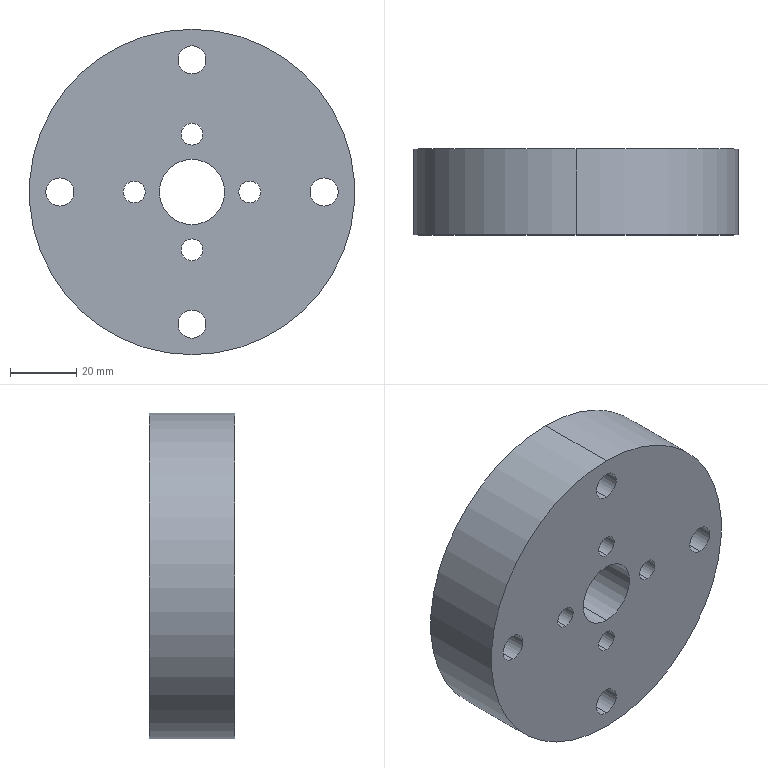Part | SolidWorks | features BaseBody 1 | 1 solid | 34 faces | box 98.5 x 26 x 98.5 mm | volume 179004 mm3 | cylinder 28 | plane 6 | commonest cylinder face diameters 6.6 x8 8.5 x8 11 x8 19.8 x2 98.5 x2
STEP:
#1=CARTESIAN_POINT('',(0.,26.,-49.25));
#2=VERTEX_POINT('',#1);
#3=CARTESIAN_POINT('',(0.,26.,49.25));
#4=VERTEX_POINT('',#3);
#5=CARTESIAN_POINT('',(0.,26.,0.));
#6=DIRECTION('',(0.,-1.,0.));
#7=DIRECTION('',(0.,0.,-1.));
#8=AXIS2_PLACEMENT_3D('',#5,#6,#7);
#9=CIRCLE('',#8,49.25);
#10=EDGE_CURVE('',#2,#4,#9,.T.);
#11=ORIENTED_EDGE('',*,*,#10,.T.);
#12=CARTESIAN_POINT('',(0.,0.,49.25));
#13=VERTEX_POINT('',#12);
#14=CARTESIAN_POINT('',(0.,26.,49.25));
#15=DIRECTION('',(0.,-1.,0.));
#16=VECTOR('',#15,1000.);
#17=LINE('',#14,#16);
#18=EDGE_CURVE('',#4,#13,#17,.T.);
#19=ORIENTED_EDGE('',*,*,#18,.T.);
#20=CARTESIAN_POINT('',(0.,0.,-49.25));
#21=VERTEX_POINT('',#20);
#22=CARTESIAN_POINT('',(0.,0.,0.));
#23=DIRECTION('',(0.,1.,0.));
#24=DIRECTION('',(0.,0.,-1.));
#25=AXIS2_PLACEMENT_3D('',#22,#23,#24);
#26=CIRCLE('',#25,49.25);
#27=EDGE_CURVE('',#13,#21,#26,.T.);
#28=ORIENTED_EDGE('',*,*,#27,.T.);
#29=CARTESIAN_POINT('',(0.,26.,-49.25));
#30=DIRECTION('',(0.,-1.,0.));
#31=VECTOR('',#30,1000.);
#32=LINE('',#29,#31);
#33=EDGE_CURVE('',#2,#21,#32,.T.);
#34=ORIENTED_EDGE('',*,*,#33,.F.);
#35=EDGE_LOOP('',(#11,#19,#28,#34));
#36=FACE_OUTER_BOUND('',#35,.T.);
#37=CARTESIAN_POINT('',(0.,26.,0.));
#38=DIRECTION('',(0.,-1.,0.));
#39=DIRECTION('',(0.,0.,-1.));
#40=AXIS2_PLACEMENT_3D('',#37,#38,#39);
#41=CYLINDRICAL_SURFACE('',#40,49.25);
#42=ADVANCED_FACE('',(#36),#41,.T.);
#43=CARTESIAN_POINT('',(0.,0.,9.9));
#44=VERTEX_POINT('',#43);
#45=CARTESIAN_POINT('',(0.,0.,-9.9));
#46=VERTEX_POINT('',#45);
#47=CARTESIAN_POINT('',(0.,0.,0.));
#48=DIRECTION('',(0.,-1.,0.));
#49=DIRECTION('',(0.,0.,1.));
#50=AXIS2_PLACEMENT_3D('',#47,#48,#49);
#51=CIRCLE('',#50,9.9);
#52=EDGE_CURVE('',#44,#46,#51,.T.);
#53=ORIENTED_EDGE('',*,*,#52,.T.);
#54=CARTESIAN_POINT('',(0.,26.,-9.9));
#55=VERTEX_POINT('',#54);
#56=CARTESIAN_POINT('',(0.,0.,-9.9));
#57=DIRECTION('',(0.,1.,0.));
#58=VECTOR('',#57,1000.);
#59=LINE('',#56,#58);
#60=EDGE_CURVE('',#46,#55,#59,.T.);
#61=ORIENTED_EDGE('',*,*,#60,.T.);
#62=CARTESIAN_POINT('',(0.,26.,9.9));
#63=VERTEX_POINT('',#62);
#64=CARTESIAN_POINT('',(0.,26.,0.));
#65=DIRECTION('',(0.,-1.,0.));
#66=DIRECTION('',(0.,0.,1.));
#67=AXIS2_PLACEMENT_3D('',#64,#65,#66);
#68=CIRCLE('',#67,9.9);
#69=EDGE_CURVE('',#63,#55,#68,.T.);
#70=ORIENTED_EDGE('',*,*,#69,.F.);
#71=CARTESIAN_POINT('',(0.,0.,9.9));
#72=DIRECTION('',(0.,1.,0.));
#73=VECTOR('',#72,1000.);
#74=LINE('',#71,#73);
#75=EDGE_CURVE('',#44,#63,#74,.T.);
#76=ORIENTED_EDGE('',*,*,#75,.F.);
#77=EDGE_LOOP('',(#53,#61,#70,#76));
#78=FACE_OUTER_BOUND('',#77,.T.);
#79=CARTESIAN_POINT('',(0.,0.,0.));
#80=DIRECTION('',(0.,1.,0.));
#81=DIRECTION('',(0.,0.,1.));
#82=AXIS2_PLACEMENT_3D('',#79,#80,#81);
#83=CYLINDRICAL_SURFACE('',#82,9.9);
#84=ADVANCED_FACE('',(#78),#83,.F.);
#85=CARTESIAN_POINT('',(0.,0.,44.25));
#86=VERTEX_POINT('',#85);
#87=CARTESIAN_POINT('',(0.,0.,35.75));
#88=VERTEX_POINT('',#87);
#89=CARTESIAN_POINT('',(0.,0.,40.));
#90=DIRECTION('',(0.,-1.,0.));
#91=DIRECTION('',(0.,0.,1.));
#92=AXIS2_PLACEMENT_3D('',#89,#90,#91);
#93=CIRCLE('',#92,4.25);
#94=EDGE_CURVE('',#86,#88,#93,.T.);
#95=ORIENTED_EDGE('',*,*,#94,.T.);
#96=CARTESIAN_POINT('',(0.,26.,35.75));
#97=VERTEX_POINT('',#96);
#98=CARTESIAN_POINT('',(0.,26.,35.75));
#99=DIRECTION('',(0.,1.,0.));
#100=VECTOR('',#99,1000.);
#101=LINE('',#98,#100);
#102=EDGE_CURVE('',#88,#97,#101,.T.);
#103=ORIENTED_EDGE('',*,*,#102,.T.);
#104=CARTESIAN_POINT('',(0.,26.,44.25));
#105=VERTEX_POINT('',#104);
#106=CARTESIAN_POINT('',(0.,26.,40.));
#107=DIRECTION('',(0.,-1.,0.));
#108=DIRECTION('',(0.,0.,1.));
#109=AXIS2_PLACEMENT_3D('',#106,#107,#108);
#110=CIRCLE('',#109,4.25);
#111=EDGE_CURVE('',#105,#97,#110,.T.);
#112=ORIENTED_EDGE('',*,*,#111,.F.);
#113=CARTESIAN_POINT('',(0.,26.,44.25));
#114=DIRECTION('',(0.,1.,0.));
#115=VECTOR('',#114,1000.);
#116=LINE('',#113,#115);
#117=EDGE_CURVE('',#86,#105,#116,.T.);
#118=ORIENTED_EDGE('',*,*,#117,.F.);
#119=EDGE_LOOP('',(#95,#103,#112,#118));
#120=FACE_OUTER_BOUND('',#119,.T.);
#121=CARTESIAN_POINT('',(0.,26.,40.));
#122=DIRECTION('',(0.,1.,0.));
#123=DIRECTION('',(0.,0.,1.));
#124=AXIS2_PLACEMENT_3D('',#121,#122,#123);
#125=CYLINDRICAL_SURFACE('',#124,4.25);
#126=ADVANCED_FACE('',(#120),#125,.F.);
#127=CARTESIAN_POINT('',(-40.,0.,4.25));
#128=VERTEX_POINT('',#127);
#129=CARTESIAN_POINT('',(-40.,0.,-4.25));
#130=VERTEX_POINT('',#129);
#131=CARTESIAN_POINT('',(-40.,0.,0.));
#132=DIRECTION('',(0.,-1.,0.));
#133=DIRECTION('',(0.,0.,1.));
#134=AXIS2_PLACEMENT_3D('',#131,#132,#133);
#135=CIRCLE('',#134,4.25);
#136=EDGE_CURVE('',#128,#130,#135,.T.);
#137=ORIENTED_EDGE('',*,*,#136,.T.);
#138=CARTESIAN_POINT('',(-40.,26.,-4.25));
#139=VERTEX_POINT('',#138);
#140=CARTESIAN_POINT('',(-40.,26.,-4.25));
#141=DIRECTION('',(0.,1.,0.));
#142=VECTOR('',#141,1000.);
#143=LINE('',#140,#142);
#144=EDGE_CURVE('',#130,#139,#143,.T.);
#145=ORIENTED_EDGE('',*,*,#144,.T.);
#146=CARTESIAN_POINT('',(-40.,26.,4.25));
#147=VERTEX_POINT('',#146);
#148=CARTESIAN_POINT('',(-40.,26.,0.));
#149=DIRECTION('',(0.,-1.,0.));
#150=DIRECTION('',(0.,0.,1.));
#151=AXIS2_PLACEMENT_3D('',#148,#149,#150);
#152=CIRCLE('',#151,4.25);
#153=EDGE_CURVE('',#147,#139,#152,.T.);
#154=ORIENTED_EDGE('',*,*,#153,.F.);
#155=CARTESIAN_POINT('',(-40.,26.,4.25));
#156=DIRECTION('',(0.,1.,0.));
#157=VECTOR('',#156,1000.);
#158=LINE('',#155,#157);
#159=EDGE_CURVE('',#128,#147,#158,.T.);
#160=ORIENTED_EDGE('',*,*,#159,.F.);
#161=EDGE_LOOP('',(#137,#145,#154,#160));
#162=FACE_OUTER_BOUND('',#161,.T.);
#163=CARTESIAN_POINT('',(-40.,26.,0.));
#164=DIRECTION('',(0.,1.,0.));
#165=DIRECTION('',(0.,0.,1.));
#166=AXIS2_PLACEMENT_3D('',#163,#164,#165);
#167=CYLINDRICAL_SURFACE('',#166,4.25);
#168=ADVANCED_FACE('',(#162),#167,.F.);
#169=CARTESIAN_POINT('',(40.,0.,4.25));
#170=VERTEX_POINT('',#169);
#171=CARTESIAN_POINT('',(40.,0.,-4.25));
#172=VERTEX_POINT('',#171);
#173=CARTESIAN_POINT('',(40.,0.,0.));
#174=DIRECTION('',(0.,-1.,0.));
#175=DIRECTION('',(0.,0.,1.));
#176=AXIS2_PLACEMENT_3D('',#173,#174,#175);
#177=CIRCLE('',#176,4.25);
#178=EDGE_CURVE('',#170,#172,#177,.T.);
#179=ORIENTED_EDGE('',*,*,#178,.T.);
#180=CARTESIAN_POINT('',(40.,26.,-4.25));
#181=VERTEX_POINT('',#180);
#182=CARTESIAN_POINT('',(40.,26.,-4.25));
#183=DIRECTION('',(0.,1.,0.));
#184=VECTOR('',#183,1000.);
#185=LINE('',#182,#184);
#186=EDGE_CURVE('',#172,#181,#185,.T.);
#187=ORIENTED_EDGE('',*,*,#186,.T.);
#188=CARTESIAN_POINT('',(40.,26.,4.25));
#189=VERTEX_POINT('',#188);
#190=CARTESIAN_POINT('',(40.,26.,0.));
#191=DIRECTION('',(0.,-1.,0.));
#192=DIRECTION('',(0.,0.,1.));
#193=AXIS2_PLACEMENT_3D('',#190,#191,#192);
#194=CIRCLE('',#193,4.25);
#195=EDGE_CURVE('',#189,#181,#194,.T.);
#196=ORIENTED_EDGE('',*,*,#195,.F.);
#197=CARTESIAN_POINT('',(40.,26.,4.25));
#198=DIRECTION('',(0.,1.,0.));
#199=VECTOR('',#198,1000.);
#200=LINE('',#197,#199);
#201=EDGE_CURVE('',#170,#189,#200,.T.);
#202=ORIENTED_EDGE('',*,*,#201,.F.);
#203=EDGE_LOOP('',(#179,#187,#196,#202));
#204=FACE_OUTER_BOUND('',#203,.T.);
#205=CARTESIAN_POINT('',(40.,26.,0.));
#206=DIRECTION('',(0.,1.,0.));
#207=DIRECTION('',(0.,0.,1.));
#208=AXIS2_PLACEMENT_3D('',#205,#206,#207);
#209=CYLINDRICAL_SURFACE('',#208,4.25);
#210=ADVANCED_FACE('',(#204),#209,.F.);
#211=CARTESIAN_POINT('',(0.,0.,-35.75));
#212=VERTEX_POINT('',#211);
#213=CARTESIAN_POINT('',(0.,0.,-44.25));
#214=VERTEX_POINT('',#213);
#215=CARTESIAN_POINT('',(0.,0.,-40.));
#216=DIRECTION('',(0.,-1.,0.));
#217=DIRECTION('',(0.,0.,1.));
#218=AXIS2_PLACEMENT_3D('',#215,#216,#217);
#219=CIRCLE('',#218,4.25);
#220=EDGE_CURVE('',#212,#214,#219,.T.);
#221=ORIENTED_EDGE('',*,*,#220,.T.);
#222=CARTESIAN_POINT('',(0.,26.,-44.25));
#223=VERTEX_POINT('',#222);
#224=CARTESIAN_POINT('',(0.,26.,-44.25));
#225=DIRECTION('',(0.,1.,0.));
#226=VECTOR('',#225,1000.);
#227=LINE('',#224,#226);
#228=EDGE_CURVE('',#214,#223,#227,.T.);
#229=ORIENTED_EDGE('',*,*,#228,.T.);
#230=CARTESIAN_POINT('',(0.,26.,-35.75));
#231=VERTEX_POINT('',#230);
#232=CARTESIAN_POINT('',(0.,26.,-40.));
#233=DIRECTION('',(0.,-1.,0.));
#234=DIRECTION('',(0.,0.,1.));
#235=AXIS2_PLACEMENT_3D('',#232,#233,#234);
#236=CIRCLE('',#235,4.25);
#237=EDGE_CURVE('',#231,#223,#236,.T.);
#238=ORIENTED_EDGE('',*,*,#237,.F.);
#239=CARTESIAN_POINT('',(0.,26.,-35.75));
#240=DIRECTION('',(0.,1.,0.));
#241=VECTOR('',#240,1000.);
#242=LINE('',#239,#241);
#243=EDGE_CURVE('',#212,#231,#242,.T.);
#244=ORIENTED_EDGE('',*,*,#243,.F.);
#245=EDGE_LOOP('',(#221,#229,#238,#244));
#246=FACE_OUTER_BOUND('',#245,.T.);
#247=CARTESIAN_POINT('',(0.,26.,-40.));
#248=DIRECTION('',(0.,1.,0.));
#249=DIRECTION('',(0.,0.,1.));
#250=AXIS2_PLACEMENT_3D('',#247,#248,#249);
#251=CYLINDRICAL_SURFACE('',#250,4.25);
#252=ADVANCED_FACE('',(#246),#251,.F.);
#253=CARTESIAN_POINT('',(-17.5,0.,3.3));
#254=VERTEX_POINT('',#253);
#255=CARTESIAN_POINT('',(-17.5,0.,-3.3));
#256=VERTEX_POINT('',#255);
#257=CARTESIAN_POINT('',(-17.5,0.,0.));
#258=DIRECTION('',(0.,-1.,0.));
#259=DIRECTION('',(0.,0.,1.));
#260=AXIS2_PLACEMENT_3D('',#257,#258,#259);
#261=CIRCLE('',#260,3.3);
#262=EDGE_CURVE('',#254,#256,#261,.T.);
#263=ORIENTED_EDGE('',*,*,#262,.T.);
#264=CARTESIAN_POINT('',(-17.5,19.2,-3.3));
#265=VERTEX_POINT('',#264);
#266=CARTESIAN_POINT('',(-17.5,26.,-3.3));
#267=DIRECTION('',(0.,1.,0.));
#268=VECTOR('',#267,1000.);
#269=LINE('',#266,#268);
#270=EDGE_CURVE('',#256,#265,#269,.T.);
#271=ORIENTED_EDGE('',*,*,#270,.T.);
#272=CARTESIAN_POINT('',(-17.5,19.2,3.3));
#273=VERTEX_POINT('',#272);
#274=CARTESIAN_POINT('',(-17.5,19.2,0.));
#275=DIRECTION('',(0.,-1.,0.));
#276=DIRECTION('',(0.,0.,1.));
#277=AXIS2_PLACEMENT_3D('',#274,#275,#276);
#278=CIRCLE('',#277,3.3);
#279=EDGE_CURVE('',#273,#265,#278,.T.);
#280=ORIENTED_EDGE('',*,*,#279,.F.);
#281=CARTESIAN_POINT('',(-17.5,26.,3.3));
#282=DIRECTION('',(0.,1.,0.));
#283=VECTOR('',#282,1000.);
#284=LINE('',#281,#283);
#285=EDGE_CURVE('',#254,#273,#284,.T.);
#286=ORIENTED_EDGE('',*,*,#285,.F.);
#287=EDGE_LOOP('',(#263,#271,#280,#286));
#288=FACE_OUTER_BOUND('',#287,.T.);
#289=CARTESIAN_POINT('',(-17.5,26.,0.));
#290=DIRECTION('',(0.,1.,0.));
#291=DIRECTION('',(0.,0.,1.));
#292=AXIS2_PLACEMENT_3D('',#289,#290,#291);
#293=CYLINDRICAL_SURFACE('',#292,3.3);
#294=ADVANCED_FACE('',(#288),#293,.F.);
#295=CARTESIAN_POINT('',(0.,0.,20.8));
#296=VERTEX_POINT('',#295);
#297=CARTESIAN_POINT('',(0.,0.,14.2));
#298=VERTEX_POINT('',#297);
#299=CARTESIAN_POINT('',(0.,0.,17.5));
#300=DIRECTION('',(0.,-1.,0.));
#301=DIRECTION('',(0.,0.,1.));
#302=AXIS2_PLACEMENT_3D('',#299,#300,#301);
#303=CIRCLE('',#302,3.3);
#304=EDGE_CURVE('',#296,#298,#303,.T.);
#305=ORIENTED_EDGE('',*,*,#304,.T.);
#306=CARTESIAN_POINT('',(0.,19.2,14.2));
#307=VERTEX_POINT('',#306);
#308=CARTESIAN_POINT('',(0.,26.,14.2));
#309=DIRECTION('',(0.,1.,0.));
#310=VECTOR('',#309,1000.);
#311=LINE('',#308,#310);
#312=EDGE_CURVE('',#298,#307,#311,.T.);
#313=ORIENTED_EDGE('',*,*,#312,.T.);
#314=CARTESIAN_POINT('',(0.,19.2,20.8));
#315=VERTEX_POINT('',#314);
#316=CARTESIAN_POINT('',(0.,19.2,17.5));
#317=DIRECTION('',(0.,-1.,0.));
#318=DIRECTION('',(0.,0.,1.));
#319=AXIS2_PLACEMENT_3D('',#316,#317,#318);
#320=CIRCLE('',#319,3.3);
#321=EDGE_CURVE('',#315,#307,#320,.T.);
#322=ORIENTED_EDGE('',*,*,#321,.F.);
#323=CARTESIAN_POINT('',(0.,26.,20.8));
#324=DIRECTION('',(0.,1.,0.));
#325=VECTOR('',#324,1000.);
#326=LINE('',#323,#325);
#327=EDGE_CURVE('',#296,#315,#326,.T.);
#328=ORIENTED_EDGE('',*,*,#327,.F.);
#329=EDGE_LOOP('',(#305,#313,#322,#328));
#330=FACE_OUTER_BOUND('',#329,.T.);
#331=CARTESIAN_POINT('',(0.,26.,17.5));
#332=DIRECTION('',(0.,1.,0.));
#333=DIRECTION('',(0.,0.,1.));
#334=AXIS2_PLACEMENT_3D('',#331,#332,#333);
#335=CYLINDRICAL_SURFACE('',#334,3.3);
#336=ADVANCED_FACE('',(#330),#335,.F.);
#337=CARTESIAN_POINT('',(17.5,0.,3.3));
#338=VERTEX_POINT('',#337);
#339=CARTESIAN_POINT('',(17.5,0.,-3.3));
#340=VERTEX_POINT('',#339);
#341=CARTESIAN_POINT('',(17.5,0.,0.));
#342=DIRECTION('',(0.,-1.,0.));
#343=DIRECTION('',(0.,0.,1.));
#344=AXIS2_PLACEMENT_3D('',#341,#342,#343);
#345=CIRCLE('',#344,3.3);
#346=EDGE_CURVE('',#338,#340,#345,.T.);
#347=ORIENTED_EDGE('',*,*,#346,.T.);
#348=CARTESIAN_POINT('',(17.5,19.2,-3.3));
#349=VERTEX_POINT('',#348);
#350=CARTESIAN_POINT('',(17.5,26.,-3.3));
#351=DIRECTION('',(0.,1.,0.));
#352=VECTOR('',#351,1000.);
#353=LINE('',#350,#352);
#354=EDGE_CURVE('',#340,#349,#353,.T.);
#355=ORIENTED_EDGE('',*,*,#354,.T.);
#356=CARTESIAN_POINT('',(17.5,19.2,3.3));
#357=VERTEX_POINT('',#356);
#358=CARTESIAN_POINT('',(17.5,19.2,0.));
#359=DIRECTION('',(0.,-1.,0.));
#360=DIRECTION('',(0.,0.,1.));
#361=AXIS2_PLACEMENT_3D('',#358,#359,#360);
#362=CIRCLE('',#361,3.3);
#363=EDGE_CURVE('',#357,#349,#362,.T.);
#364=ORIENTED_EDGE('',*,*,#363,.F.);
#365=CARTESIAN_POINT('',(17.5,26.,3.3));
#366=DIRECTION('',(0.,1.,0.));
#367=VECTOR('',#366,1000.);
#368=LINE('',#365,#367);
#369=EDGE_CURVE('',#338,#357,#368,.T.);
#370=ORIENTED_EDGE('',*,*,#369,.F.);
#371=EDGE_LOOP('',(#347,#355,#364,#370));
#372=FACE_OUTER_BOUND('',#371,.T.);
#373=CARTESIAN_POINT('',(17.5,26.,0.));
#374=DIRECTION('',(0.,1.,0.));
#375=DIRECTION('',(0.,0.,1.));
#376=AXIS2_PLACEMENT_3D('',#373,#374,#375);
#377=CYLINDRICAL_SURFACE('',#376,3.3);
#378=ADVANCED_FACE('',(#372),#377,.F.);
#379=CARTESIAN_POINT('',(0.,0.,-14.2));
#380=VERTEX_POINT('',#379);
#381=CARTESIAN_POINT('',(0.,0.,-20.8));
#382=VERTEX_POINT('',#381);
#383=CARTESIAN_POINT('',(0.,0.,-17.5));
#384=DIRECTION('',(0.,-1.,0.));
#385=DIRECTION('',(0.,0.,1.));
#386=AXIS2_PLACEMENT_3D('',#383,#384,#385);
#387=CIRCLE('',#386,3.3);
#388=EDGE_CURVE('',#380,#382,#387,.T.);
#389=ORIENTED_EDGE('',*,*,#388,.T.);
#390=CARTESIAN_POINT('',(0.,19.2,-20.8));
#391=VERTEX_POINT('',#390);
#392=CARTESIAN_POINT('',(0.,26.,-20.8));
#393=DIRECTION('',(0.,1.,0.));
#394=VECTOR('',#393,1000.);
#395=LINE('',#392,#394);
#396=EDGE_CURVE('',#382,#391,#395,.T.);
#397=ORIENTED_EDGE('',*,*,#396,.T.);
#398=CARTESIAN_POINT('',(0.,19.2,-14.2));
#399=VERTEX_POINT('',#398);
#400=CARTESIAN_POINT('',(0.,19.2,-17.5));
#401=DIRECTION('',(0.,-1.,0.));
#402=DIRECTION('',(0.,0.,1.));
#403=AXIS2_PLACEMENT_3D('',#400,#401,#402);
#404=CIRCLE('',#403,3.3);
#405=EDGE_CURVE('',#399,#391,#404,.T.);
#406=ORIENTED_EDGE('',*,*,#405,.F.);
#407=CARTESIAN_POINT('',(0.,26.,-14.2));
#408=DIRECTION('',(0.,1.,0.));
#409=VECTOR('',#408,1000.);
#410=LINE('',#407,#409);
#411=EDGE_CURVE('',#380,#399,#410,.T.);
#412=ORIENTED_EDGE('',*,*,#411,.F.);
#413=EDGE_LOOP('',(#389,#397,#406,#412));
#414=FACE_OUTER_BOUND('',#413,.T.);
#415=CARTESIAN_POINT('',(0.,26.,-17.5));
#416=DIRECTION('',(0.,1.,0.));
#417=DIRECTION('',(0.,0.,1.));
#418=AXIS2_PLACEMENT_3D('',#415,#416,#417);
#419=CYLINDRICAL_SURFACE('',#418,3.3);
#420=ADVANCED_FACE('',(#414),#419,.F.);
#421=CARTESIAN_POINT('',(-17.5,19.2,5.5));
#422=VERTEX_POINT('',#421);
#423=CARTESIAN_POINT('',(-17.5,19.2,-5.5));
#424=VERTEX_POINT('',#423);
#425=CARTESIAN_POINT('',(-17.5,19.2,0.));
#426=DIRECTION('',(0.,-1.,0.));
#427=DIRECTION('',(0.,0.,1.));
#428=AXIS2_PLACEMENT_3D('',#425,#426,#427);
#429=CIRCLE('',#428,5.5);
#430=EDGE_CURVE('',#422,#424,#429,.T.);
#431=ORIENTED_EDGE('',*,*,#430,.T.);
#432=CARTESIAN_POINT('',(-17.5,26.,-5.5));
#433=VERTEX_POINT('',#432);
#434=CARTESIAN_POINT('',(-17.5,26.,-5.5));
#435=DIRECTION('',(0.,1.,0.));
#436=VECTOR('',#435,1000.);
#437=LINE('',#434,#436);
#438=EDGE_CURVE('',#424,#433,#437,.T.);
#439=ORIENTED_EDGE('',*,*,#438,.T.);
#440=CARTESIAN_POINT('',(-17.5,26.,5.5));
#441=VERTEX_POINT('',#440);
#442=CARTESIAN_POINT('',(-17.5,26.,0.));
#443=DIRECTION('',(0.,-1.,0.));
#444=DIRECTION('',(0.,0.,1.));
#445=AXIS2_PLACEMENT_3D('',#442,#443,#444);
#446=CIRCLE('',#445,5.5);
#447=EDGE_CURVE('',#441,#433,#446,.T.);
#448=ORIENTED_EDGE('',*,*,#447,.F.);
#449=CARTESIAN_POINT('',(-17.5,26.,5.5));
#450=DIRECTION('',(0.,1.,0.));
#451=VECTOR('',#450,1000.);
#452=LINE('',#449,#451);
#453=EDGE_CURVE('',#422,#441,#452,.T.);
#454=ORIENTED_EDGE('',*,*,#453,.F.);
#455=EDGE_LOOP('',(#431,#439,#448,#454));
#456=FACE_OUTER_BOUND('',#455,.T.);
#457=CARTESIAN_POINT('',(-17.5,26.,0.));
#458=DIRECTION('',(0.,1.,0.));
#459=DIRECTION('',(0.,0.,1.));
#460=AXIS2_PLACEMENT_3D('',#457,#458,#459);
#461=CYLINDRICAL_SURFACE('',#460,5.5);
#462=ADVANCED_FACE('',(#456),#461,.F.);
#463=CARTESIAN_POINT('',(0.,19.2,23.));
#464=VERTEX_POINT('',#463);
#465=CARTESIAN_POINT('',(0.,19.2,12.));
#466=VERTEX_POINT('',#465);
#467=CARTESIAN_POINT('',(0.,19.2,17.5));
#468=DIRECTION('',(0.,-1.,0.));
#469=DIRECTION('',(0.,0.,1.));
#470=AXIS2_PLACEMENT_3D('',#467,#468,#469);
#471=CIRCLE('',#470,5.5);
#472=EDGE_CURVE('',#464,#466,#471,.T.);
#473=ORIENTED_EDGE('',*,*,#472,.T.);
#474=CARTESIAN_POINT('',(0.,26.,12.));
#475=VERTEX_POINT('',#474);
#476=CARTESIAN_POINT('',(0.,26.,12.));
#477=DIRECTION('',(0.,1.,0.));
#478=VECTOR('',#477,1000.);
#479=LINE('',#476,#478);
#480=EDGE_CURVE('',#466,#475,#479,.T.);
#481=ORIENTED_EDGE('',*,*,#480,.T.);
#482=CARTESIAN_POINT('',(0.,26.,23.));
#483=VERTEX_POINT('',#482);
#484=CARTESIAN_POINT('',(0.,26.,17.5));
#485=DIRECTION('',(0.,-1.,0.));
#486=DIRECTION('',(0.,0.,1.));
#487=AXIS2_PLACEMENT_3D('',#484,#485,#486);
#488=CIRCLE('',#487,5.5);
#489=EDGE_CURVE('',#483,#475,#488,.T.);
#490=ORIENTED_EDGE('',*,*,#489,.F.);
#491=CARTESIAN_POINT('',(0.,26.,23.));
#492=DIRECTION('',(0.,1.,0.));
#493=VECTOR('',#492,1000.);
#494=LINE('',#491,#493);
#495=EDGE_CURVE('',#464,#483,#494,.T.);
#496=ORIENTED_EDGE('',*,*,#495,.F.);
#497=EDGE_LOOP('',(#473,#481,#490,#496));
#498=FACE_OUTER_BOUND('',#497,.T.);
#499=CARTESIAN_POINT('',(0.,26.,17.5));
#500=DIRECTION('',(0.,1.,0.));
#501=DIRECTION('',(0.,0.,1.));
#502=AXIS2_PLACEMENT_3D('',#499,#500,#501);
#503=CYLINDRICAL_SURFACE('',#502,5.5);
#504=ADVANCED_FACE('',(#498),#503,.F.);
#505=CARTESIAN_POINT('',(17.5,19.2,5.5));
#506=VERTEX_POINT('',#505);
#507=CARTESIAN_POINT('',(17.5,19.2,-5.5));
#508=VERTEX_POINT('',#507);
#509=CARTESIAN_POINT('',(17.5,19.2,0.));
#510=DIRECTION('',(0.,-1.,0.));
#511=DIRECTION('',(0.,0.,1.));
#512=AXIS2_PLACEMENT_3D('',#509,#510,#511);
#513=CIRCLE('',#512,5.5);
#514=EDGE_CURVE('',#506,#508,#513,.T.);
#515=ORIENTED_EDGE('',*,*,#514,.T.);
#516=CARTESIAN_POINT('',(17.5,26.,-5.5));
#517=VERTEX_POINT('',#516);
#518=CARTESIAN_POINT('',(17.5,26.,-5.5));
#519=DIRECTION('',(0.,1.,0.));
#520=VECTOR('',#519,1000.);
#521=LINE('',#518,#520);
#522=EDGE_CURVE('',#508,#517,#521,.T.);
#523=ORIENTED_EDGE('',*,*,#522,.T.);
#524=CARTESIAN_POINT('',(17.5,26.,5.5));
#525=VERTEX_POINT('',#524);
#526=CARTESIAN_POINT('',(17.5,26.,0.));
#527=DIRECTION('',(0.,-1.,0.));
#528=DIRECTION('',(0.,0.,1.));
#529=AXIS2_PLACEMENT_3D('',#526,#527,#528);
#530=CIRCLE('',#529,5.5);
#531=EDGE_CURVE('',#525,#517,#530,.T.);
#532=ORIENTED_EDGE('',*,*,#531,.F.);
#533=CARTESIAN_POINT('',(17.5,26.,5.5));
#534=DIRECTION('',(0.,1.,0.));
#535=VECTOR('',#534,1000.);
#536=LINE('',#533,#535);
#537=EDGE_CURVE('',#506,#525,#536,.T.);
#538=ORIENTED_EDGE('',*,*,#537,.F.);
#539=EDGE_LOOP('',(#515,#523,#532,#538));
#540=FACE_OUTER_BOUND('',#539,.T.);
#541=CARTESIAN_POINT('',(17.5,26.,0.));
#542=DIRECTION('',(0.,1.,0.));
#543=DIRECTION('',(0.,0.,1.));
#544=AXIS2_PLACEMENT_3D('',#541,#542,#543);
#545=CYLINDRICAL_SURFACE('',#544,5.5);
#546=ADVANCED_FACE('',(#540),#545,.F.);
#547=CARTESIAN_POINT('',(0.,19.2,-12.));
#548=VERTEX_POINT('',#547);
#549=CARTESIAN_POINT('',(0.,19.2,-23.));
#550=VERTEX_POINT('',#549);
#551=CARTESIAN_POINT('',(0.,19.2,-17.5));
#552=DIRECTION('',(0.,-1.,0.));
#553=DIRECTION('',(0.,0.,1.));
#554=AXIS2_PLACEMENT_3D('',#551,#552,#553);
#555=CIRCLE('',#554,5.5);
#556=EDGE_CURVE('',#548,#550,#555,.T.);
#557=ORIENTED_EDGE('',*,*,#556,.T.);
#558=CARTESIAN_POINT('',(0.,26.,-23.));
#559=VERTEX_POINT('',#558);
#560=CARTESIAN_POINT('',(0.,26.,-23.));
#561=DIRECTION('',(0.,1.,0.));
#562=VECTOR('',#561,1000.);
#563=LINE('',#560,#562);
#564=EDGE_CURVE('',#550,#559,#563,.T.);
#565=ORIENTED_EDGE('',*,*,#564,.T.);
#566=CARTESIAN_POINT('',(0.,26.,-12.));
#567=VERTEX_POINT('',#566);
#568=CARTESIAN_POINT('',(0.,26.,-17.5));
#569=DIRECTION('',(0.,-1.,0.));
#570=DIRECTION('',(0.,0.,1.));
#571=AXIS2_PLACEMENT_3D('',#568,#569,#570);
#572=CIRCLE('',#571,5.5);
#573=EDGE_CURVE('',#567,#559,#572,.T.);
#574=ORIENTED_EDGE('',*,*,#573,.F.);
#575=CARTESIAN_POINT('',(0.,26.,-12.));
#576=DIRECTION('',(0.,1.,0.));
#577=VECTOR('',#576,1000.);
#578=LINE('',#575,#577);
#579=EDGE_CURVE('',#548,#567,#578,.T.);
#580=ORIENTED_EDGE('',*,*,#579,.F.);
#581=EDGE_LOOP('',(#557,#565,#574,#580));
#582=FACE_OUTER_BOUND('',#581,.T.);
#583=CARTESIAN_POINT('',(0.,26.,-17.5));
#584=DIRECTION('',(0.,1.,0.));
#585=DIRECTION('',(0.,0.,1.));
#586=AXIS2_PLACEMENT_3D('',#583,#584,#585);
#587=CYLINDRICAL_SURFACE('',#586,5.5);
#588=ADVANCED_FACE('',(#582),#587,.F.);
#589=CARTESIAN_POINT('',(0.,0.,0.));
#590=DIRECTION('',(0.,1.,0.));
#591=DIRECTION('',(0.,0.,-1.));
#592=AXIS2_PLACEMENT_3D('',#589,#590,#591);
#593=CIRCLE('',#592,49.25);
#594=EDGE_CURVE('',#21,#13,#593,.T.);
#595=ORIENTED_EDGE('',*,*,#594,.F.);
#596=ORIENTED_EDGE('',*,*,#27,.F.);
#597=EDGE_LOOP('',(#595,#596));
#598=FACE_OUTER_BOUND('',#597,.T.);
#599=ORIENTED_EDGE('',*,*,#52,.F.);
#600=CARTESIAN_POINT('',(0.,0.,0.));
#601=DIRECTION('',(0.,-1.,0.));
#602=DIRECTION('',(0.,0.,1.));
#603=AXIS2_PLACEMENT_3D('',#600,#601,#602);
#604=CIRCLE('',#603,9.9);
#605=EDGE_CURVE('',#46,#44,#604,.T.);
#606=ORIENTED_EDGE('',*,*,#605,.F.);
#607=EDGE_LOOP('',(#599,#606));
#608=FACE_BOUND('',#607,.T.);
#609=ORIENTED_EDGE('',*,*,#94,.F.);
#610=CARTESIAN_POINT('',(0.,0.,40.));
#611=DIRECTION('',(0.,-1.,0.));
#612=DIRECTION('',(0.,0.,1.));
#613=AXIS2_PLACEMENT_3D('',#610,#611,#612);
#614=CIRCLE('',#613,4.25);
#615=EDGE_CURVE('',#88,#86,#614,.T.);
#616=ORIENTED_EDGE('',*,*,#615,.F.);
#617=EDGE_LOOP('',(#609,#616));
#618=FACE_BOUND('',#617,.T.);
#619=ORIENTED_EDGE('',*,*,#136,.F.);
#620=CARTESIAN_POINT('',(-40.,0.,0.));
#621=DIRECTION('',(0.,-1.,0.));
#622=DIRECTION('',(0.,0.,1.));
#623=AXIS2_PLACEMENT_3D('',#620,#621,#622);
#624=CIRCLE('',#623,4.25);
#625=EDGE_CURVE('',#130,#128,#624,.T.);
#626=ORIENTED_EDGE('',*,*,#625,.F.);
#627=EDGE_LOOP('',(#619,#626));
#628=FACE_BOUND('',#627,.T.);
#629=ORIENTED_EDGE('',*,*,#178,.F.);
#630=CARTESIAN_POINT('',(40.,0.,0.));
#631=DIRECTION('',(0.,-1.,0.));
#632=DIRECTION('',(0.,0.,1.));
#633=AXIS2_PLACEMENT_3D('',#630,#631,#632);
#634=CIRCLE('',#633,4.25);
#635=EDGE_CURVE('',#172,#170,#634,.T.);
#636=ORIENTED_EDGE('',*,*,#635,.F.);
#637=EDGE_LOOP('',(#629,#636));
#638=FACE_BOUND('',#637,.T.);
#639=ORIENTED_EDGE('',*,*,#220,.F.);
#640=CARTESIAN_POINT('',(0.,0.,-40.));
#641=DIRECTION('',(0.,-1.,0.));
#642=DIRECTION('',(0.,0.,1.));
#643=AXIS2_PLACEMENT_3D('',#640,#641,#642);
#644=CIRCLE('',#643,4.25);
#645=EDGE_CURVE('',#214,#212,#644,.T.);
#646=ORIENTED_EDGE('',*,*,#645,.F.);
#647=EDGE_LOOP('',(#639,#646));
#648=FACE_BOUND('',#647,.T.);
#649=ORIENTED_EDGE('',*,*,#262,.F.);
#650=CARTESIAN_POINT('',(-17.5,0.,0.));
#651=DIRECTION('',(0.,-1.,0.));
#652=DIRECTION('',(0.,0.,1.));
#653=AXIS2_PLACEMENT_3D('',#650,#651,#652);
#654=CIRCLE('',#653,3.3);
#655=EDGE_CURVE('',#256,#254,#654,.T.);
#656=ORIENTED_EDGE('',*,*,#655,.F.);
#657=EDGE_LOOP('',(#649,#656));
#658=FACE_BOUND('',#657,.T.);
#659=ORIENTED_EDGE('',*,*,#304,.F.);
#660=CARTESIAN_POINT('',(0.,0.,17.5));
#661=DIRECTION('',(0.,-1.,0.));
#662=DIRECTION('',(0.,0.,1.));
#663=AXIS2_PLACEMENT_3D('',#660,#661,#662);
#664=CIRCLE('',#663,3.3);
#665=EDGE_CURVE('',#298,#296,#664,.T.);
#666=ORIENTED_EDGE('',*,*,#665,.F.);
#667=EDGE_LOOP('',(#659,#666));
#668=FACE_BOUND('',#667,.T.);
#669=ORIENTED_EDGE('',*,*,#346,.F.);
#670=CARTESIAN_POINT('',(17.5,0.,0.));
#671=DIRECTION('',(0.,-1.,0.));
#672=DIRECTION('',(0.,0.,1.));
#673=AXIS2_PLACEMENT_3D('',#670,#671,#672);
#674=CIRCLE('',#673,3.3);
#675=EDGE_CURVE('',#340,#338,#674,.T.);
#676=ORIENTED_EDGE('',*,*,#675,.F.);
#677=EDGE_LOOP('',(#669,#676));
#678=FACE_BOUND('',#677,.T.);
#679=ORIENTED_EDGE('',*,*,#388,.F.);
#680=CARTESIAN_POINT('',(0.,0.,-17.5));
#681=DIRECTION('',(0.,-1.,0.));
#682=DIRECTION('',(0.,0.,1.));
#683=AXIS2_PLACEMENT_3D('',#680,#681,#682);
#684=CIRCLE('',#683,3.3);
#685=EDGE_CURVE('',#382,#380,#684,.T.);
#686=ORIENTED_EDGE('',*,*,#685,.F.);
#687=EDGE_LOOP('',(#679,#686));
#688=FACE_BOUND('',#687,.T.);
#689=CARTESIAN_POINT('',(0.,0.,0.));
#690=DIRECTION('',(0.,1.,0.));
#691=DIRECTION('',(0.,0.,1.));
#692=AXIS2_PLACEMENT_3D('',#689,#690,#691);
#693=PLANE('',#692);
#694=ADVANCED_FACE('',(#598,#608,#618,#628,#638,#648,#658,#668,#678,#688),#693,.F.);
#695=ORIENTED_EDGE('',*,*,#18,.F.);
#696=CARTESIAN_POINT('',(0.,26.,0.));
#697=DIRECTION('',(0.,-1.,0.));
#698=DIRECTION('',(0.,0.,-1.));
#699=AXIS2_PLACEMENT_3D('',#696,#697,#698);
#700=CIRCLE('',#699,49.25);
#701=EDGE_CURVE('',#4,#2,#700,.T.);
#702=ORIENTED_EDGE('',*,*,#701,.T.);
#703=ORIENTED_EDGE('',*,*,#33,.T.);
#704=ORIENTED_EDGE('',*,*,#594,.T.);
#705=EDGE_LOOP('',(#695,#702,#703,#704));
#706=FACE_OUTER_BOUND('',#705,.T.);
#707=CARTESIAN_POINT('',(0.,26.,0.));
#708=DIRECTION('',(0.,-1.,0.));
#709=DIRECTION('',(0.,0.,-1.));
#710=AXIS2_PLACEMENT_3D('',#707,#708,#709);
#711=CYLINDRICAL_SURFACE('',#710,49.25);
#712=ADVANCED_FACE('',(#706),#711,.T.);
#713=ORIENTED_EDGE('',*,*,#60,.F.);
#714=ORIENTED_EDGE('',*,*,#605,.T.);
#715=ORIENTED_EDGE('',*,*,#75,.T.);
#716=CARTESIAN_POINT('',(0.,26.,0.));
#717=DIRECTION('',(0.,-1.,0.));
#718=DIRECTION('',(0.,0.,1.));
#719=AXIS2_PLACEMENT_3D('',#716,#717,#718);
#720=CIRCLE('',#719,9.9);
#721=EDGE_CURVE('',#55,#63,#720,.T.);
#722=ORIENTED_EDGE('',*,*,#721,.F.);
#723=EDGE_LOOP('',(#713,#714,#715,#722));
#724=FACE_OUTER_BOUND('',#723,.T.);
#725=CARTESIAN_POINT('',(0.,0.,0.));
#726=DIRECTION('',(0.,1.,0.));
#727=DIRECTION('',(0.,0.,1.));
#728=AXIS2_PLACEMENT_3D('',#725,#726,#727);
#729=CYLINDRICAL_SURFACE('',#728,9.9);
#730=ADVANCED_FACE('',(#724),#729,.F.);
#731=ORIENTED_EDGE('',*,*,#102,.F.);
#732=ORIENTED_EDGE('',*,*,#615,.T.);
#733=ORIENTED_EDGE('',*,*,#117,.T.);
#734=CARTESIAN_POINT('',(0.,26.,40.));
#735=DIRECTION('',(0.,-1.,0.));
#736=DIRECTION('',(0.,0.,1.));
#737=AXIS2_PLACEMENT_3D('',#734,#735,#736);
#738=CIRCLE('',#737,4.25);
#739=EDGE_CURVE('',#97,#105,#738,.T.);
#740=ORIENTED_EDGE('',*,*,#739,.F.);
#741=EDGE_LOOP('',(#731,#732,#733,#740));
#742=FACE_OUTER_BOUND('',#741,.T.);
#743=CARTESIAN_POINT('',(0.,26.,40.));
#744=DIRECTION('',(0.,1.,0.));
#745=DIRECTION('',(0.,0.,1.));
#746=AXIS2_PLACEMENT_3D('',#743,#744,#745);
#747=CYLINDRICAL_SURFACE('',#746,4.25);
#748=ADVANCED_FACE('',(#742),#747,.F.);
#749=ORIENTED_EDGE('',*,*,#144,.F.);
#750=ORIENTED_EDGE('',*,*,#625,.T.);
#751=ORIENTED_EDGE('',*,*,#159,.T.);
#752=CARTESIAN_POINT('',(-40.,26.,0.));
#753=DIRECTION('',(0.,-1.,0.));
#754=DIRECTION('',(0.,0.,1.));
#755=AXIS2_PLACEMENT_3D('',#752,#753,#754);
#756=CIRCLE('',#755,4.25);
#757=EDGE_CURVE('',#139,#147,#756,.T.);
#758=ORIENTED_EDGE('',*,*,#757,.F.);
#759=EDGE_LOOP('',(#749,#750,#751,#758));
#760=FACE_OUTER_BOUND('',#759,.T.);
#761=CARTESIAN_POINT('',(-40.,26.,0.));
#762=DIRECTION('',(0.,1.,0.));
#763=DIRECTION('',(0.,0.,1.));
#764=AXIS2_PLACEMENT_3D('',#761,#762,#763);
#765=CYLINDRICAL_SURFACE('',#764,4.25);
#766=ADVANCED_FACE('',(#760),#765,.F.);
#767=ORIENTED_EDGE('',*,*,#186,.F.);
#768=ORIENTED_EDGE('',*,*,#635,.T.);
#769=ORIENTED_EDGE('',*,*,#201,.T.);
#770=CARTESIAN_POINT('',(40.,26.,0.));
#771=DIRECTION('',(0.,-1.,0.));
#772=DIRECTION('',(0.,0.,1.));
#773=AXIS2_PLACEMENT_3D('',#770,#771,#772);
#774=CIRCLE('',#773,4.25);
#775=EDGE_CURVE('',#181,#189,#774,.T.);
#776=ORIENTED_EDGE('',*,*,#775,.F.);
#777=EDGE_LOOP('',(#767,#768,#769,#776));
#778=FACE_OUTER_BOUND('',#777,.T.);
#779=CARTESIAN_POINT('',(40.,26.,0.));
#780=DIRECTION('',(0.,1.,0.));
#781=DIRECTION('',(0.,0.,1.));
#782=AXIS2_PLACEMENT_3D('',#779,#780,#781);
#783=CYLINDRICAL_SURFACE('',#782,4.25);
#784=ADVANCED_FACE('',(#778),#783,.F.);
#785=ORIENTED_EDGE('',*,*,#228,.F.);
#786=ORIENTED_EDGE('',*,*,#645,.T.);
#787=ORIENTED_EDGE('',*,*,#243,.T.);
#788=CARTESIAN_POINT('',(0.,26.,-40.));
#789=DIRECTION('',(0.,-1.,0.));
#790=DIRECTION('',(0.,0.,1.));
#791=AXIS2_PLACEMENT_3D('',#788,#789,#790);
#792=CIRCLE('',#791,4.25);
#793=EDGE_CURVE('',#223,#231,#792,.T.);
#794=ORIENTED_EDGE('',*,*,#793,.F.);
#795=EDGE_LOOP('',(#785,#786,#787,#794));
#796=FACE_OUTER_BOUND('',#795,.T.);
#797=CARTESIAN_POINT('',(0.,26.,-40.));
#798=DIRECTION('',(0.,1.,0.));
#799=DIRECTION('',(0.,0.,1.));
#800=AXIS2_PLACEMENT_3D('',#797,#798,#799);
#801=CYLINDRICAL_SURFACE('',#800,4.25);
#802=ADVANCED_FACE('',(#796),#801,.F.);
#803=ORIENTED_EDGE('',*,*,#270,.F.);
#804=ORIENTED_EDGE('',*,*,#655,.T.);
#805=ORIENTED_EDGE('',*,*,#285,.T.);
#806=CARTESIAN_POINT('',(-17.5,19.2,0.));
#807=DIRECTION('',(0.,-1.,0.));
#808=DIRECTION('',(0.,0.,1.));
#809=AXIS2_PLACEMENT_3D('',#806,#807,#808);
#810=CIRCLE('',#809,3.3);
#811=EDGE_CURVE('',#265,#273,#810,.T.);
#812=ORIENTED_EDGE('',*,*,#811,.F.);
#813=EDGE_LOOP('',(#803,#804,#805,#812));
#814=FACE_OUTER_BOUND('',#813,.T.);
#815=CARTESIAN_POINT('',(-17.5,26.,0.));
#816=DIRECTION('',(0.,1.,0.));
#817=DIRECTION('',(0.,0.,1.));
#818=AXIS2_PLACEMENT_3D('',#815,#816,#817);
#819=CYLINDRICAL_SURFACE('',#818,3.3);
#820=ADVANCED_FACE('',(#814),#819,.F.);
#821=ORIENTED_EDGE('',*,*,#312,.F.);
#822=ORIENTED_EDGE('',*,*,#665,.T.);
#823=ORIENTED_EDGE('',*,*,#327,.T.);
#824=CARTESIAN_POINT('',(0.,19.2,17.5));
#825=DIRECTION('',(0.,-1.,0.));
#826=DIRECTION('',(0.,0.,1.));
#827=AXIS2_PLACEMENT_3D('',#824,#825,#826);
#828=CIRCLE('',#827,3.3);
#829=EDGE_CURVE('',#307,#315,#828,.T.);
#830=ORIENTED_EDGE('',*,*,#829,.F.);
#831=EDGE_LOOP('',(#821,#822,#823,#830));
#832=FACE_OUTER_BOUND('',#831,.T.);
#833=CARTESIAN_POINT('',(0.,26.,17.5));
#834=DIRECTION('',(0.,1.,0.));
#835=DIRECTION('',(0.,0.,1.));
#836=AXIS2_PLACEMENT_3D('',#833,#834,#835);
#837=CYLINDRICAL_SURFACE('',#836,3.3);
#838=ADVANCED_FACE('',(#832),#837,.F.);
#839=ORIENTED_EDGE('',*,*,#354,.F.);
#840=ORIENTED_EDGE('',*,*,#675,.T.);
#841=ORIENTED_EDGE('',*,*,#369,.T.);
#842=CARTESIAN_POINT('',(17.5,19.2,0.));
#843=DIRECTION('',(0.,-1.,0.));
#844=DIRECTION('',(0.,0.,1.));
#845=AXIS2_PLACEMENT_3D('',#842,#843,#844);
#846=CIRCLE('',#845,3.3);
#847=EDGE_CURVE('',#349,#357,#846,.T.);
#848=ORIENTED_EDGE('',*,*,#847,.F.);
#849=EDGE_LOOP('',(#839,#840,#841,#848));
#850=FACE_OUTER_BOUND('',#849,.T.);
#851=CARTESIAN_POINT('',(17.5,26.,0.));
#852=DIRECTION('',(0.,1.,0.));
#853=DIRECTION('',(0.,0.,1.));
#854=AXIS2_PLACEMENT_3D('',#851,#852,#853);
#855=CYLINDRICAL_SURFACE('',#854,3.3);
#856=ADVANCED_FACE('',(#850),#855,.F.);
#857=ORIENTED_EDGE('',*,*,#396,.F.);
#858=ORIENTED_EDGE('',*,*,#685,.T.);
#859=ORIENTED_EDGE('',*,*,#411,.T.);
#860=CARTESIAN_POINT('',(0.,19.2,-17.5));
#861=DIRECTION('',(0.,-1.,0.));
#862=DIRECTION('',(0.,0.,1.));
#863=AXIS2_PLACEMENT_3D('',#860,#861,#862);
#864=CIRCLE('',#863,3.3);
#865=EDGE_CURVE('',#391,#399,#864,.T.);
#866=ORIENTED_EDGE('',*,*,#865,.F.);
#867=EDGE_LOOP('',(#857,#858,#859,#866));
#868=FACE_OUTER_BOUND('',#867,.T.);
#869=CARTESIAN_POINT('',(0.,26.,-17.5));
#870=DIRECTION('',(0.,1.,0.));
#871=DIRECTION('',(0.,0.,1.));
#872=AXIS2_PLACEMENT_3D('',#869,#870,#871);
#873=CYLINDRICAL_SURFACE('',#872,3.3);
#874=ADVANCED_FACE('',(#868),#873,.F.);
#875=ORIENTED_EDGE('',*,*,#10,.F.);
#876=ORIENTED_EDGE('',*,*,#701,.F.);
#877=EDGE_LOOP('',(#875,#876));
#878=FACE_OUTER_BOUND('',#877,.T.);
#879=ORIENTED_EDGE('',*,*,#69,.T.);
#880=ORIENTED_EDGE('',*,*,#721,.T.);
#881=EDGE_LOOP('',(#879,#880));
#882=FACE_BOUND('',#881,.T.);
#883=ORIENTED_EDGE('',*,*,#111,.T.);
#884=ORIENTED_EDGE('',*,*,#739,.T.);
#885=EDGE_LOOP('',(#883,#884));
#886=FACE_BOUND('',#885,.T.);
#887=ORIENTED_EDGE('',*,*,#153,.T.);
#888=ORIENTED_EDGE('',*,*,#757,.T.);
#889=EDGE_LOOP('',(#887,#888));
#890=FACE_BOUND('',#889,.T.);
#891=ORIENTED_EDGE('',*,*,#195,.T.);
#892=ORIENTED_EDGE('',*,*,#775,.T.);
#893=EDGE_LOOP('',(#891,#892));
#894=FACE_BOUND('',#893,.T.);
#895=ORIENTED_EDGE('',*,*,#237,.T.);
#896=ORIENTED_EDGE('',*,*,#793,.T.);
#897=EDGE_LOOP('',(#895,#896));
#898=FACE_BOUND('',#897,.T.);
#899=ORIENTED_EDGE('',*,*,#447,.T.);
#900=CARTESIAN_POINT('',(-17.5,26.,0.));
#901=DIRECTION('',(0.,-1.,0.));
#902=DIRECTION('',(0.,0.,1.));
#903=AXIS2_PLACEMENT_3D('',#900,#901,#902);
#904=CIRCLE('',#903,5.5);
#905=EDGE_CURVE('',#433,#441,#904,.T.);
#906=ORIENTED_EDGE('',*,*,#905,.T.);
#907=EDGE_LOOP('',(#899,#906));
#908=FACE_BOUND('',#907,.T.);
#909=ORIENTED_EDGE('',*,*,#489,.T.);
#910=CARTESIAN_POINT('',(0.,26.,17.5));
#911=DIRECTION('',(0.,-1.,0.));
#912=DIRECTION('',(0.,0.,1.));
#913=AXIS2_PLACEMENT_3D('',#910,#911,#912);
#914=CIRCLE('',#913,5.5);
#915=EDGE_CURVE('',#475,#483,#914,.T.);
#916=ORIENTED_EDGE('',*,*,#915,.T.);
#917=EDGE_LOOP('',(#909,#916));
#918=FACE_BOUND('',#917,.T.);
#919=ORIENTED_EDGE('',*,*,#531,.T.);
#920=CARTESIAN_POINT('',(17.5,26.,0.));
#921=DIRECTION('',(0.,-1.,0.));
#922=DIRECTION('',(0.,0.,1.));
#923=AXIS2_PLACEMENT_3D('',#920,#921,#922);
#924=CIRCLE('',#923,5.5);
#925=EDGE_CURVE('',#517,#525,#924,.T.);
#926=ORIENTED_EDGE('',*,*,#925,.T.);
#927=EDGE_LOOP('',(#919,#926));
#928=FACE_BOUND('',#927,.T.);
#929=ORIENTED_EDGE('',*,*,#573,.T.);
#930=CARTESIAN_POINT('',(0.,26.,-17.5));
#931=DIRECTION('',(0.,-1.,0.));
#932=DIRECTION('',(0.,0.,1.));
#933=AXIS2_PLACEMENT_3D('',#930,#931,#932);
#934=CIRCLE('',#933,5.5);
#935=EDGE_CURVE('',#559,#567,#934,.T.);
#936=ORIENTED_EDGE('',*,*,#935,.T.);
#937=EDGE_LOOP('',(#929,#936));
#938=FACE_BOUND('',#937,.T.);
#939=CARTESIAN_POINT('',(0.,26.,0.));
#940=DIRECTION('',(0.,1.,0.));
#941=DIRECTION('',(0.,0.,1.));
#942=AXIS2_PLACEMENT_3D('',#939,#940,#941);
#943=PLANE('',#942);
#944=ADVANCED_FACE('',(#878,#882,#886,#890,#894,#898,#908,#918,#928,#938),#943,.T.);
#945=ORIENTED_EDGE('',*,*,#430,.F.);
#946=CARTESIAN_POINT('',(-17.5,19.2,0.));
#947=DIRECTION('',(0.,-1.,0.));
#948=DIRECTION('',(0.,0.,1.));
#949=AXIS2_PLACEMENT_3D('',#946,#947,#948);
#950=CIRCLE('',#949,5.5);
#951=EDGE_CURVE('',#424,#422,#950,.T.);
#952=ORIENTED_EDGE('',*,*,#951,.F.);
#953=EDGE_LOOP('',(#945,#952));
#954=FACE_OUTER_BOUND('',#953,.T.);
#955=ORIENTED_EDGE('',*,*,#279,.T.);
#956=ORIENTED_EDGE('',*,*,#811,.T.);
#957=EDGE_LOOP('',(#955,#956));
#958=FACE_BOUND('',#957,.T.);
#959=CARTESIAN_POINT('',(-14.2,19.2,0.));
#960=DIRECTION('',(0.,-1.,0.));
#961=DIRECTION('',(0.,0.,-1.));
#962=AXIS2_PLACEMENT_3D('',#959,#960,#961);
#963=PLANE('',#962);
#964=ADVANCED_FACE('',(#954,#958),#963,.F.);
#965=ORIENTED_EDGE('',*,*,#472,.F.);
#966=CARTESIAN_POINT('',(0.,19.2,17.5));
#967=DIRECTION('',(0.,-1.,0.));
#968=DIRECTION('',(0.,0.,1.));
#969=AXIS2_PLACEMENT_3D('',#966,#967,#968);
#970=CIRCLE('',#969,5.5);
#971=EDGE_CURVE('',#466,#464,#970,.T.);
#972=ORIENTED_EDGE('',*,*,#971,.F.);
#973=EDGE_LOOP('',(#965,#972));
#974=FACE_OUTER_BOUND('',#973,.T.);
#975=ORIENTED_EDGE('',*,*,#321,.T.);
#976=ORIENTED_EDGE('',*,*,#829,.T.);
#977=EDGE_LOOP('',(#975,#976));
#978=FACE_BOUND('',#977,.T.);
#979=CARTESIAN_POINT('',(3.3,19.2,17.5));
#980=DIRECTION('',(0.,-1.,0.));
#981=DIRECTION('',(0.,0.,-1.));
#982=AXIS2_PLACEMENT_3D('',#979,#980,#981);
#983=PLANE('',#982);
#984=ADVANCED_FACE('',(#974,#978),#983,.F.);
#985=ORIENTED_EDGE('',*,*,#514,.F.);
#986=CARTESIAN_POINT('',(17.5,19.2,0.));
#987=DIRECTION('',(0.,-1.,0.));
#988=DIRECTION('',(0.,0.,1.));
#989=AXIS2_PLACEMENT_3D('',#986,#987,#988);
#990=CIRCLE('',#989,5.5);
#991=EDGE_CURVE('',#508,#506,#990,.T.);
#992=ORIENTED_EDGE('',*,*,#991,.F.);
#993=EDGE_LOOP('',(#985,#992));
#994=FACE_OUTER_BOUND('',#993,.T.);
#995=ORIENTED_EDGE('',*,*,#363,.T.);
#996=ORIENTED_EDGE('',*,*,#847,.T.);
#997=EDGE_LOOP('',(#995,#996));
#998=FACE_BOUND('',#997,.T.);
#999=CARTESIAN_POINT('',(20.8,19.2,0.));
#1000=DIRECTION('',(0.,-1.,0.));
#1001=DIRECTION('',(0.,0.,-1.));
#1002=AXIS2_PLACEMENT_3D('',#999,#1000,#1001);
#1003=PLANE('',#1002);
#1004=ADVANCED_FACE('',(#994,#998),#1003,.F.);
#1005=ORIENTED_EDGE('',*,*,#556,.F.);
#1006=CARTESIAN_POINT('',(0.,19.2,-17.5));
#1007=DIRECTION('',(0.,-1.,0.));
#1008=DIRECTION('',(0.,0.,1.));
#1009=AXIS2_PLACEMENT_3D('',#1006,#1007,#1008);
#1010=CIRCLE('',#1009,5.5);
#1011=EDGE_CURVE('',#550,#548,#1010,.T.);
#1012=ORIENTED_EDGE('',*,*,#1011,.F.);
#1013=EDGE_LOOP('',(#1005,#1012));
#1014=FACE_OUTER_BOUND('',#1013,.T.);
#1015=ORIENTED_EDGE('',*,*,#405,.T.);
#1016=ORIENTED_EDGE('',*,*,#865,.T.);
#1017=EDGE_LOOP('',(#1015,#1016));
#1018=FACE_BOUND('',#1017,.T.);
#1019=CARTESIAN_POINT('',(3.3,19.2,-17.5));
#1020=DIRECTION('',(0.,-1.,0.));
#1021=DIRECTION('',(0.,0.,-1.));
#1022=AXIS2_PLACEMENT_3D('',#1019,#1020,#1021);
#1023=PLANE('',#1022);
#1024=ADVANCED_FACE('',(#1014,#1018),#1023,.F.);
#1025=ORIENTED_EDGE('',*,*,#438,.F.);
#1026=ORIENTED_EDGE('',*,*,#951,.T.);
#1027=ORIENTED_EDGE('',*,*,#453,.T.);
#1028=ORIENTED_EDGE('',*,*,#905,.F.);
#1029=EDGE_LOOP('',(#1025,#1026,#1027,#1028));
#1030=FACE_OUTER_BOUND('',#1029,.T.);
#1031=CARTESIAN_POINT('',(-17.5,26.,0.));
#1032=DIRECTION('',(0.,1.,0.));
#1033=DIRECTION('',(0.,0.,1.));
#1034=AXIS2_PLACEMENT_3D('',#1031,#1032,#1033);
#1035=CYLINDRICAL_SURFACE('',#1034,5.5);
#1036=ADVANCED_FACE('',(#1030),#1035,.F.);
#1037=ORIENTED_EDGE('',*,*,#480,.F.);
#1038=ORIENTED_EDGE('',*,*,#971,.T.);
#1039=ORIENTED_EDGE('',*,*,#495,.T.);
#1040=ORIENTED_EDGE('',*,*,#915,.F.);
#1041=EDGE_LOOP('',(#1037,#1038,#1039,#1040));
#1042=FACE_OUTER_BOUND('',#1041,.T.);
#1043=CARTESIAN_POINT('',(0.,26.,17.5));
#1044=DIRECTION('',(0.,1.,0.));
#1045=DIRECTION('',(0.,0.,1.));
#1046=AXIS2_PLACEMENT_3D('',#1043,#1044,#1045);
#1047=CYLINDRICAL_SURFACE('',#1046,5.5);
#1048=ADVANCED_FACE('',(#1042),#1047,.F.);
#1049=ORIENTED_EDGE('',*,*,#522,.F.);
#1050=ORIENTED_EDGE('',*,*,#991,.T.);
#1051=ORIENTED_EDGE('',*,*,#537,.T.);
#1052=ORIENTED_EDGE('',*,*,#925,.F.);
#1053=EDGE_LOOP('',(#1049,#1050,#1051,#1052));
#1054=FACE_OUTER_BOUND('',#1053,.T.);
#1055=CARTESIAN_POINT('',(17.5,26.,0.));
#1056=DIRECTION('',(0.,1.,0.));
#1057=DIRECTION('',(0.,0.,1.));
#1058=AXIS2_PLACEMENT_3D('',#1055,#1056,#1057);
#1059=CYLINDRICAL_SURFACE('',#1058,5.5);
#1060=ADVANCED_FACE('',(#1054),#1059,.F.);
#1061=ORIENTED_EDGE('',*,*,#564,.F.);
#1062=ORIENTED_EDGE('',*,*,#1011,.T.);
#1063=ORIENTED_EDGE('',*,*,#579,.T.);
#1064=ORIENTED_EDGE('',*,*,#935,.F.);
#1065=EDGE_LOOP('',(#1061,#1062,#1063,#1064));
#1066=FACE_OUTER_BOUND('',#1065,.T.);
#1067=CARTESIAN_POINT('',(0.,26.,-17.5));
#1068=DIRECTION('',(0.,1.,0.));
#1069=DIRECTION('',(0.,0.,1.));
#1070=AXIS2_PLACEMENT_3D('',#1067,#1068,#1069);
#1071=CYLINDRICAL_SURFACE('',#1070,5.5);
#1072=ADVANCED_FACE('',(#1066),#1071,.F.);
#1073=CLOSED_SHELL('',(#42,#84,#126,#168,#210,#252,#294,#336,#378,#420,#462,#504,#546,#588,#694,#712,#730,#748,#766,#784,#802,#820,#838,#856,#874,#944,#964,#984,#1004,#1024,#1036,#1048,#1060,#1072));
#1074=MANIFOLD_SOLID_BREP('',#1073);
#1075=CARTESIAN_POINT('',(0.,0.,0.));
#1076=DIRECTION('',(0.,0.,1.));
#1077=DIRECTION('',(1.,0.,0.));
#1078=AXIS2_PLACEMENT_3D('',#1075,#1076,#1077);
#1079=(LENGTH_UNIT()NAMED_UNIT(*)SI_UNIT(.MILLI.,.METRE.));
#1080=UNCERTAINTY_MEASURE_WITH_UNIT(LENGTH_MEASURE(0.00001),#1079,'','');
#1081=(NAMED_UNIT(*)PLANE_ANGLE_UNIT()SI_UNIT($,.RADIAN.));
#1082=(NAMED_UNIT(*)SI_UNIT($,.STERADIAN.)SOLID_ANGLE_UNIT());
#1083=(GEOMETRIC_REPRESENTATION_CONTEXT(3)GLOBAL_UNCERTAINTY_ASSIGNED_CONTEXT((#1080))GLOBAL_UNIT_ASSIGNED_CONTEXT((#1079,#1081,#1082))REPRESENTATION_CONTEXT('',''));
#1084=ADVANCED_BREP_SHAPE_REPRESENTATION('',(#1074,#1078),#1083);